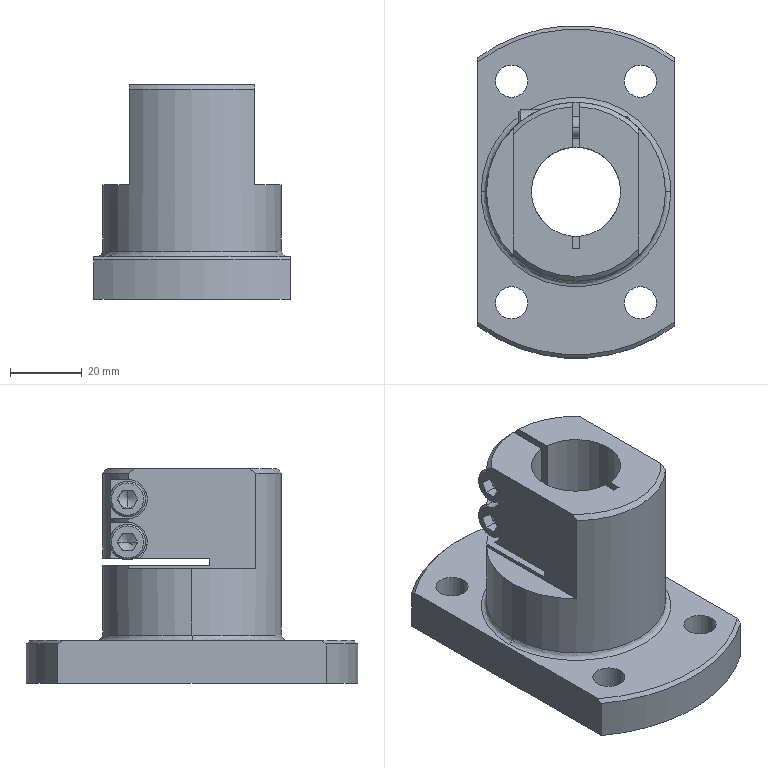Part | SolidWorks | features BaseBody 1 | 1 solid | 122 faces | box 55 x 93 x 60 mm | volume 106506 mm3 | plane 59 | cylinder 40 | cone 21 | spline 2 | commonest cylinder face diameters 9 x8 4.917 x6 6 x6 6.6 x4 10 x4 25 x4